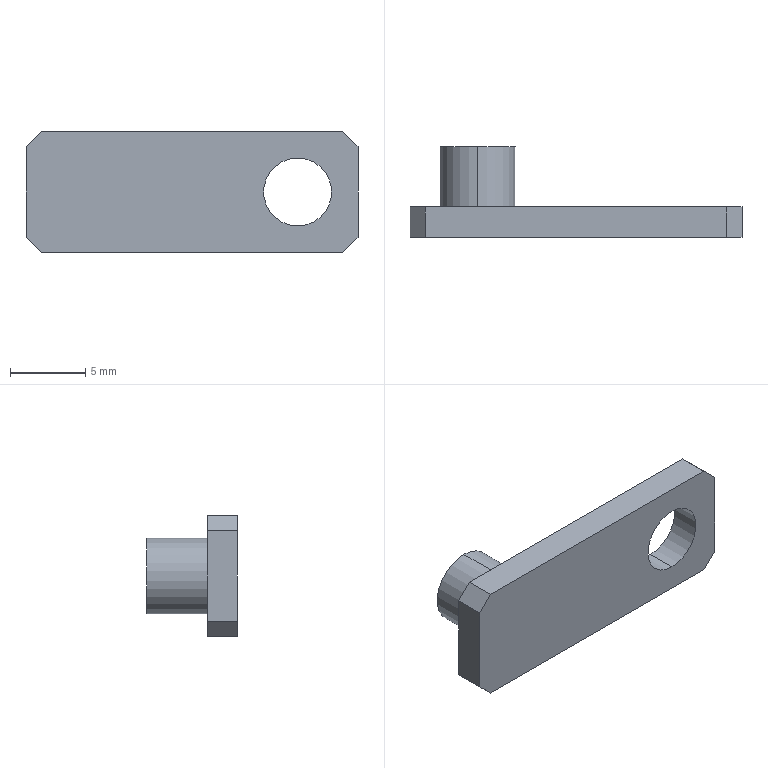Part | SolidWorks | features ICE 2, Chamfer 1, Extrusion 1 | 1 solid | 15 faces | box 22 x 6 x 8 mm | volume 394.731 mm3 | plane 11 | cylinder 4 | commonest cylinder face diameters 4.5 x2 5 x2
STEP:
#1=CARTESIAN_POINT('',(-6.5,6.,2.5));
#2=VERTEX_POINT('',#1);
#3=CARTESIAN_POINT('',(-6.5,6.,-2.5));
#4=VERTEX_POINT('',#3);
#5=CARTESIAN_POINT('',(-6.5,6.,0.));
#6=DIRECTION('',(0.,1.,0.));
#7=DIRECTION('',(0.,0.,1.));
#8=AXIS2_PLACEMENT_3D('',#5,#6,#7);
#9=CIRCLE('',#8,2.5);
#10=EDGE_CURVE('',#2,#4,#9,.T.);
#11=ORIENTED_EDGE('',*,*,#10,.F.);
#12=CARTESIAN_POINT('',(-6.5,2.,2.5));
#13=VERTEX_POINT('',#12);
#14=CARTESIAN_POINT('',(-6.5,6.,2.5));
#15=DIRECTION('',(0.,-1.,0.));
#16=VECTOR('',#15,1000.);
#17=LINE('',#14,#16);
#18=EDGE_CURVE('',#2,#13,#17,.T.);
#19=ORIENTED_EDGE('',*,*,#18,.T.);
#20=CARTESIAN_POINT('',(-6.5,2.,-2.5));
#21=VERTEX_POINT('',#20);
#22=CARTESIAN_POINT('',(-6.5,2.,0.));
#23=DIRECTION('',(0.,1.,0.));
#24=DIRECTION('',(0.,0.,-1.));
#25=AXIS2_PLACEMENT_3D('',#22,#23,#24);
#26=CIRCLE('',#25,2.5);
#27=EDGE_CURVE('',#13,#21,#26,.T.);
#28=ORIENTED_EDGE('',*,*,#27,.T.);
#29=CARTESIAN_POINT('',(-6.5,6.,-2.5));
#30=DIRECTION('',(0.,-1.,0.));
#31=VECTOR('',#30,1000.);
#32=LINE('',#29,#31);
#33=EDGE_CURVE('',#4,#21,#32,.T.);
#34=ORIENTED_EDGE('',*,*,#33,.F.);
#35=EDGE_LOOP('',(#11,#19,#28,#34));
#36=FACE_OUTER_BOUND('',#35,.T.);
#37=CARTESIAN_POINT('',(-6.5,6.,0.));
#38=DIRECTION('',(0.,-1.,0.));
#39=DIRECTION('',(0.,0.,-1.));
#40=AXIS2_PLACEMENT_3D('',#37,#38,#39);
#41=CYLINDRICAL_SURFACE('',#40,2.5);
#42=ADVANCED_FACE('',(#36),#41,.T.);
#43=CARTESIAN_POINT('',(7.,0.,-2.25));
#44=VERTEX_POINT('',#43);
#45=CARTESIAN_POINT('',(7.,0.,2.25));
#46=VERTEX_POINT('',#45);
#47=CARTESIAN_POINT('',(7.,0.,0.));
#48=DIRECTION('',(0.,1.,0.));
#49=DIRECTION('',(0.,0.,1.));
#50=AXIS2_PLACEMENT_3D('',#47,#48,#49);
#51=CIRCLE('',#50,2.25);
#52=EDGE_CURVE('',#44,#46,#51,.T.);
#53=ORIENTED_EDGE('',*,*,#52,.F.);
#54=CARTESIAN_POINT('',(7.,2.,-2.25));
#55=VERTEX_POINT('',#54);
#56=CARTESIAN_POINT('',(7.,0.,-2.25));
#57=DIRECTION('',(0.,1.,0.));
#58=VECTOR('',#57,1000.);
#59=LINE('',#56,#58);
#60=EDGE_CURVE('',#44,#55,#59,.T.);
#61=ORIENTED_EDGE('',*,*,#60,.T.);
#62=CARTESIAN_POINT('',(7.,2.,2.25));
#63=VERTEX_POINT('',#62);
#64=CARTESIAN_POINT('',(7.,2.,0.));
#65=DIRECTION('',(0.,1.,0.));
#66=DIRECTION('',(0.,0.,1.));
#67=AXIS2_PLACEMENT_3D('',#64,#65,#66);
#68=CIRCLE('',#67,2.25);
#69=EDGE_CURVE('',#55,#63,#68,.T.);
#70=ORIENTED_EDGE('',*,*,#69,.T.);
#71=CARTESIAN_POINT('',(7.,0.,2.25));
#72=DIRECTION('',(0.,1.,0.));
#73=VECTOR('',#72,1000.);
#74=LINE('',#71,#73);
#75=EDGE_CURVE('',#46,#63,#74,.T.);
#76=ORIENTED_EDGE('',*,*,#75,.F.);
#77=EDGE_LOOP('',(#53,#61,#70,#76));
#78=FACE_OUTER_BOUND('',#77,.T.);
#79=CARTESIAN_POINT('',(7.,0.,0.));
#80=DIRECTION('',(0.,1.,0.));
#81=DIRECTION('',(0.,0.,1.));
#82=AXIS2_PLACEMENT_3D('',#79,#80,#81);
#83=CYLINDRICAL_SURFACE('',#82,2.25);
#84=ADVANCED_FACE('',(#78),#83,.F.);
#85=CARTESIAN_POINT('',(11.,0.,3.));
#86=VERTEX_POINT('',#85);
#87=CARTESIAN_POINT('',(11.,0.,-3.));
#88=VERTEX_POINT('',#87);
#89=CARTESIAN_POINT('',(11.,0.,4.));
#90=DIRECTION('',(0.,0.,-1.));
#91=VECTOR('',#90,1000.);
#92=LINE('',#89,#91);
#93=EDGE_CURVE('',#86,#88,#92,.T.);
#94=ORIENTED_EDGE('',*,*,#93,.T.);
#95=CARTESIAN_POINT('',(11.,2.,-3.));
#96=VERTEX_POINT('',#95);
#97=CARTESIAN_POINT('',(11.,2.,-3.));
#98=DIRECTION('',(0.,1.,0.));
#99=VECTOR('',#98,1000.);
#100=LINE('',#97,#99);
#101=EDGE_CURVE('',#88,#96,#100,.T.);
#102=ORIENTED_EDGE('',*,*,#101,.T.);
#103=CARTESIAN_POINT('',(11.,2.,3.));
#104=VERTEX_POINT('',#103);
#105=CARTESIAN_POINT('',(11.,2.,4.));
#106=DIRECTION('',(0.,0.,-1.));
#107=VECTOR('',#106,1000.);
#108=LINE('',#105,#107);
#109=EDGE_CURVE('',#104,#96,#108,.T.);
#110=ORIENTED_EDGE('',*,*,#109,.F.);
#111=CARTESIAN_POINT('',(11.,2.,3.));
#112=DIRECTION('',(0.,-1.,0.));
#113=VECTOR('',#112,1000.);
#114=LINE('',#111,#113);
#115=EDGE_CURVE('',#104,#86,#114,.T.);
#116=ORIENTED_EDGE('',*,*,#115,.T.);
#117=EDGE_LOOP('',(#94,#102,#110,#116));
#118=FACE_OUTER_BOUND('',#117,.T.);
#119=CARTESIAN_POINT('',(11.,2.,4.));
#120=DIRECTION('',(-1.,0.,0.));
#121=DIRECTION('',(0.,0.,1.));
#122=AXIS2_PLACEMENT_3D('',#119,#120,#121);
#123=PLANE('',#122);
#124=ADVANCED_FACE('',(#118),#123,.F.);
#125=CARTESIAN_POINT('',(10.,2.,-4.));
#126=VERTEX_POINT('',#125);
#127=CARTESIAN_POINT('',(-10.,2.,-4.));
#128=VERTEX_POINT('',#127);
#129=CARTESIAN_POINT('',(-11.,2.,-4.));
#130=DIRECTION('',(-1.,0.,0.));
#131=VECTOR('',#130,1000.);
#132=LINE('',#129,#131);
#133=EDGE_CURVE('',#126,#128,#132,.T.);
#134=ORIENTED_EDGE('',*,*,#133,.F.);
#135=CARTESIAN_POINT('',(10.,0.,-4.));
#136=VERTEX_POINT('',#135);
#137=CARTESIAN_POINT('',(10.,2.,-4.));
#138=DIRECTION('',(0.,-1.,0.));
#139=VECTOR('',#138,1000.);
#140=LINE('',#137,#139);
#141=EDGE_CURVE('',#126,#136,#140,.T.);
#142=ORIENTED_EDGE('',*,*,#141,.T.);
#143=CARTESIAN_POINT('',(-10.,0.,-4.));
#144=VERTEX_POINT('',#143);
#145=CARTESIAN_POINT('',(-11.,0.,-4.));
#146=DIRECTION('',(-1.,0.,0.));
#147=VECTOR('',#146,1000.);
#148=LINE('',#145,#147);
#149=EDGE_CURVE('',#136,#144,#148,.T.);
#150=ORIENTED_EDGE('',*,*,#149,.T.);
#151=CARTESIAN_POINT('',(-10.,2.,-4.));
#152=DIRECTION('',(0.,1.,0.));
#153=VECTOR('',#152,1000.);
#154=LINE('',#151,#153);
#155=EDGE_CURVE('',#144,#128,#154,.T.);
#156=ORIENTED_EDGE('',*,*,#155,.T.);
#157=EDGE_LOOP('',(#134,#142,#150,#156));
#158=FACE_OUTER_BOUND('',#157,.T.);
#159=CARTESIAN_POINT('',(-11.,2.,-4.));
#160=DIRECTION('',(0.,0.,1.));
#161=DIRECTION('',(1.,0.,0.));
#162=AXIS2_PLACEMENT_3D('',#159,#160,#161);
#163=PLANE('',#162);
#164=ADVANCED_FACE('',(#158),#163,.F.);
#165=CARTESIAN_POINT('',(-11.,2.,-3.));
#166=VERTEX_POINT('',#165);
#167=CARTESIAN_POINT('',(-11.,2.,3.));
#168=VERTEX_POINT('',#167);
#169=CARTESIAN_POINT('',(-11.,2.,4.));
#170=DIRECTION('',(0.,0.,1.));
#171=VECTOR('',#170,1000.);
#172=LINE('',#169,#171);
#173=EDGE_CURVE('',#166,#168,#172,.T.);
#174=ORIENTED_EDGE('',*,*,#173,.F.);
#175=CARTESIAN_POINT('',(-11.,0.,-3.));
#176=VERTEX_POINT('',#175);
#177=CARTESIAN_POINT('',(-11.,2.,-3.));
#178=DIRECTION('',(0.,-1.,0.));
#179=VECTOR('',#178,1000.);
#180=LINE('',#177,#179);
#181=EDGE_CURVE('',#166,#176,#180,.T.);
#182=ORIENTED_EDGE('',*,*,#181,.T.);
#183=CARTESIAN_POINT('',(-11.,0.,3.));
#184=VERTEX_POINT('',#183);
#185=CARTESIAN_POINT('',(-11.,0.,4.));
#186=DIRECTION('',(0.,0.,1.));
#187=VECTOR('',#186,1000.);
#188=LINE('',#185,#187);
#189=EDGE_CURVE('',#176,#184,#188,.T.);
#190=ORIENTED_EDGE('',*,*,#189,.T.);
#191=CARTESIAN_POINT('',(-11.,2.,3.));
#192=DIRECTION('',(0.,1.,0.));
#193=VECTOR('',#192,1000.);
#194=LINE('',#191,#193);
#195=EDGE_CURVE('',#184,#168,#194,.T.);
#196=ORIENTED_EDGE('',*,*,#195,.T.);
#197=EDGE_LOOP('',(#174,#182,#190,#196));
#198=FACE_OUTER_BOUND('',#197,.T.);
#199=CARTESIAN_POINT('',(-11.,2.,4.));
#200=DIRECTION('',(1.,0.,0.));
#201=DIRECTION('',(0.,0.,-1.));
#202=AXIS2_PLACEMENT_3D('',#199,#200,#201);
#203=PLANE('',#202);
#204=ADVANCED_FACE('',(#198),#203,.F.);
#205=CARTESIAN_POINT('',(-10.,0.,4.));
#206=VERTEX_POINT('',#205);
#207=CARTESIAN_POINT('',(10.,0.,4.));
#208=VERTEX_POINT('',#207);
#209=CARTESIAN_POINT('',(-11.,0.,4.));
#210=DIRECTION('',(1.,0.,0.));
#211=VECTOR('',#210,1000.);
#212=LINE('',#209,#211);
#213=EDGE_CURVE('',#206,#208,#212,.T.);
#214=ORIENTED_EDGE('',*,*,#213,.T.);
#215=CARTESIAN_POINT('',(10.,2.,4.));
#216=VERTEX_POINT('',#215);
#217=CARTESIAN_POINT('',(10.,2.,4.));
#218=DIRECTION('',(0.,1.,0.));
#219=VECTOR('',#218,1000.);
#220=LINE('',#217,#219);
#221=EDGE_CURVE('',#208,#216,#220,.T.);
#222=ORIENTED_EDGE('',*,*,#221,.T.);
#223=CARTESIAN_POINT('',(-10.,2.,4.));
#224=VERTEX_POINT('',#223);
#225=CARTESIAN_POINT('',(-11.,2.,4.));
#226=DIRECTION('',(1.,0.,0.));
#227=VECTOR('',#226,1000.);
#228=LINE('',#225,#227);
#229=EDGE_CURVE('',#224,#216,#228,.T.);
#230=ORIENTED_EDGE('',*,*,#229,.F.);
#231=CARTESIAN_POINT('',(-10.,2.,4.));
#232=DIRECTION('',(0.,-1.,0.));
#233=VECTOR('',#232,1000.);
#234=LINE('',#231,#233);
#235=EDGE_CURVE('',#224,#206,#234,.T.);
#236=ORIENTED_EDGE('',*,*,#235,.T.);
#237=EDGE_LOOP('',(#214,#222,#230,#236));
#238=FACE_OUTER_BOUND('',#237,.T.);
#239=CARTESIAN_POINT('',(-11.,2.,4.));
#240=DIRECTION('',(0.,0.,-1.));
#241=DIRECTION('',(-1.,0.,0.));
#242=AXIS2_PLACEMENT_3D('',#239,#240,#241);
#243=PLANE('',#242);
#244=ADVANCED_FACE('',(#238),#243,.F.);
#245=CARTESIAN_POINT('',(-6.5,2.,0.));
#246=DIRECTION('',(0.,1.,0.));
#247=DIRECTION('',(0.,0.,-1.));
#248=AXIS2_PLACEMENT_3D('',#245,#246,#247);
#249=CIRCLE('',#248,2.5);
#250=EDGE_CURVE('',#21,#13,#249,.T.);
#251=ORIENTED_EDGE('',*,*,#250,.F.);
#252=ORIENTED_EDGE('',*,*,#27,.F.);
#253=EDGE_LOOP('',(#251,#252));
#254=FACE_BOUND('',#253,.T.);
#255=CARTESIAN_POINT('',(7.,2.,0.));
#256=DIRECTION('',(0.,1.,0.));
#257=DIRECTION('',(0.,0.,1.));
#258=AXIS2_PLACEMENT_3D('',#255,#256,#257);
#259=CIRCLE('',#258,2.25);
#260=EDGE_CURVE('',#63,#55,#259,.T.);
#261=ORIENTED_EDGE('',*,*,#260,.F.);
#262=ORIENTED_EDGE('',*,*,#69,.F.);
#263=EDGE_LOOP('',(#261,#262));
#264=FACE_BOUND('',#263,.T.);
#265=ORIENTED_EDGE('',*,*,#109,.T.);
#266=CARTESIAN_POINT('',(10.,2.,-4.));
#267=DIRECTION('',(-0.7071,0.,-0.7071));
#268=VECTOR('',#267,1000.);
#269=LINE('',#266,#268);
#270=EDGE_CURVE('',#96,#126,#269,.T.);
#271=ORIENTED_EDGE('',*,*,#270,.T.);
#272=ORIENTED_EDGE('',*,*,#133,.T.);
#273=CARTESIAN_POINT('',(-11.,2.,-3.));
#274=DIRECTION('',(-0.7071,0.,0.7071));
#275=VECTOR('',#274,1000.);
#276=LINE('',#273,#275);
#277=EDGE_CURVE('',#128,#166,#276,.T.);
#278=ORIENTED_EDGE('',*,*,#277,.T.);
#279=ORIENTED_EDGE('',*,*,#173,.T.);
#280=CARTESIAN_POINT('',(-10.,2.,4.));
#281=DIRECTION('',(0.7071,0.,0.7071));
#282=VECTOR('',#281,1000.);
#283=LINE('',#280,#282);
#284=EDGE_CURVE('',#168,#224,#283,.T.);
#285=ORIENTED_EDGE('',*,*,#284,.T.);
#286=ORIENTED_EDGE('',*,*,#229,.T.);
#287=CARTESIAN_POINT('',(11.,2.,3.));
#288=DIRECTION('',(0.7071,0.,-0.7071));
#289=VECTOR('',#288,1000.);
#290=LINE('',#287,#289);
#291=EDGE_CURVE('',#216,#104,#290,.T.);
#292=ORIENTED_EDGE('',*,*,#291,.T.);
#293=EDGE_LOOP('',(#265,#271,#272,#278,#279,#285,#286,#292));
#294=FACE_OUTER_BOUND('',#293,.T.);
#295=CARTESIAN_POINT('',(0.,2.,0.));
#296=DIRECTION('',(0.,-1.,0.));
#297=DIRECTION('',(0.,0.,-1.));
#298=AXIS2_PLACEMENT_3D('',#295,#296,#297);
#299=PLANE('',#298);
#300=ADVANCED_FACE('',(#254,#264,#294),#299,.F.);
#301=CARTESIAN_POINT('',(7.,0.,0.));
#302=DIRECTION('',(0.,1.,0.));
#303=DIRECTION('',(0.,0.,1.));
#304=AXIS2_PLACEMENT_3D('',#301,#302,#303);
#305=CIRCLE('',#304,2.25);
#306=EDGE_CURVE('',#46,#44,#305,.T.);
#307=ORIENTED_EDGE('',*,*,#306,.T.);
#308=ORIENTED_EDGE('',*,*,#52,.T.);
#309=EDGE_LOOP('',(#307,#308));
#310=FACE_BOUND('',#309,.T.);
#311=ORIENTED_EDGE('',*,*,#149,.F.);
#312=CARTESIAN_POINT('',(7.,0.,-7.));
#313=DIRECTION('',(0.7071,0.,0.7071));
#314=VECTOR('',#313,1000.);
#315=LINE('',#312,#314);
#316=EDGE_CURVE('',#136,#88,#315,.T.);
#317=ORIENTED_EDGE('',*,*,#316,.T.);
#318=ORIENTED_EDGE('',*,*,#93,.F.);
#319=CARTESIAN_POINT('',(7.,0.,7.));
#320=DIRECTION('',(-0.7071,0.,0.7071));
#321=VECTOR('',#320,1000.);
#322=LINE('',#319,#321);
#323=EDGE_CURVE('',#86,#208,#322,.T.);
#324=ORIENTED_EDGE('',*,*,#323,.T.);
#325=ORIENTED_EDGE('',*,*,#213,.F.);
#326=CARTESIAN_POINT('',(-7.,0.,7.));
#327=DIRECTION('',(-0.7071,0.,-0.7071));
#328=VECTOR('',#327,1000.);
#329=LINE('',#326,#328);
#330=EDGE_CURVE('',#206,#184,#329,.T.);
#331=ORIENTED_EDGE('',*,*,#330,.T.);
#332=ORIENTED_EDGE('',*,*,#189,.F.);
#333=CARTESIAN_POINT('',(-7.,0.,-7.));
#334=DIRECTION('',(0.7071,0.,-0.7071));
#335=VECTOR('',#334,1000.);
#336=LINE('',#333,#335);
#337=EDGE_CURVE('',#176,#144,#336,.T.);
#338=ORIENTED_EDGE('',*,*,#337,.T.);
#339=EDGE_LOOP('',(#311,#317,#318,#324,#325,#331,#332,#338));
#340=FACE_OUTER_BOUND('',#339,.T.);
#341=CARTESIAN_POINT('',(0.,0.,0.));
#342=DIRECTION('',(0.,-1.,0.));
#343=DIRECTION('',(0.,0.,-1.));
#344=AXIS2_PLACEMENT_3D('',#341,#342,#343);
#345=PLANE('',#344);
#346=ADVANCED_FACE('',(#310,#340),#345,.T.);
#347=ORIENTED_EDGE('',*,*,#60,.F.);
#348=ORIENTED_EDGE('',*,*,#306,.F.);
#349=ORIENTED_EDGE('',*,*,#75,.T.);
#350=ORIENTED_EDGE('',*,*,#260,.T.);
#351=EDGE_LOOP('',(#347,#348,#349,#350));
#352=FACE_OUTER_BOUND('',#351,.T.);
#353=CARTESIAN_POINT('',(7.,0.,0.));
#354=DIRECTION('',(0.,1.,0.));
#355=DIRECTION('',(0.,0.,1.));
#356=AXIS2_PLACEMENT_3D('',#353,#354,#355);
#357=CYLINDRICAL_SURFACE('',#356,2.25);
#358=ADVANCED_FACE('',(#352),#357,.F.);
#359=ORIENTED_EDGE('',*,*,#18,.F.);
#360=CARTESIAN_POINT('',(-6.5,6.,0.));
#361=DIRECTION('',(0.,1.,0.));
#362=DIRECTION('',(0.,0.,1.));
#363=AXIS2_PLACEMENT_3D('',#360,#361,#362);
#364=CIRCLE('',#363,2.5);
#365=EDGE_CURVE('',#4,#2,#364,.T.);
#366=ORIENTED_EDGE('',*,*,#365,.F.);
#367=ORIENTED_EDGE('',*,*,#33,.T.);
#368=ORIENTED_EDGE('',*,*,#250,.T.);
#369=EDGE_LOOP('',(#359,#366,#367,#368));
#370=FACE_OUTER_BOUND('',#369,.T.);
#371=CARTESIAN_POINT('',(-6.5,6.,0.));
#372=DIRECTION('',(0.,-1.,0.));
#373=DIRECTION('',(0.,0.,-1.));
#374=AXIS2_PLACEMENT_3D('',#371,#372,#373);
#375=CYLINDRICAL_SURFACE('',#374,2.5);
#376=ADVANCED_FACE('',(#370),#375,.T.);
#377=ORIENTED_EDGE('',*,*,#365,.T.);
#378=ORIENTED_EDGE('',*,*,#10,.T.);
#379=EDGE_LOOP('',(#377,#378));
#380=FACE_OUTER_BOUND('',#379,.T.);
#381=CARTESIAN_POINT('',(-6.5,6.,0.));
#382=DIRECTION('',(0.,1.,0.));
#383=DIRECTION('',(0.,0.,1.));
#384=AXIS2_PLACEMENT_3D('',#381,#382,#383);
#385=PLANE('',#384);
#386=ADVANCED_FACE('',(#380),#385,.T.);
#387=ORIENTED_EDGE('',*,*,#270,.F.);
#388=ORIENTED_EDGE('',*,*,#101,.F.);
#389=ORIENTED_EDGE('',*,*,#316,.F.);
#390=ORIENTED_EDGE('',*,*,#141,.F.);
#391=EDGE_LOOP('',(#387,#388,#389,#390));
#392=FACE_OUTER_BOUND('',#391,.T.);
#393=CARTESIAN_POINT('',(10.,2.,-4.));
#394=DIRECTION('',(-0.7071,0.,0.7071));
#395=DIRECTION('',(0.,-1.,0.));
#396=AXIS2_PLACEMENT_3D('',#393,#394,#395);
#397=PLANE('',#396);
#398=ADVANCED_FACE('',(#392),#397,.F.);
#399=ORIENTED_EDGE('',*,*,#291,.F.);
#400=ORIENTED_EDGE('',*,*,#221,.F.);
#401=ORIENTED_EDGE('',*,*,#323,.F.);
#402=ORIENTED_EDGE('',*,*,#115,.F.);
#403=EDGE_LOOP('',(#399,#400,#401,#402));
#404=FACE_OUTER_BOUND('',#403,.T.);
#405=CARTESIAN_POINT('',(11.,2.,3.));
#406=DIRECTION('',(-0.7071,0.,-0.7071));
#407=DIRECTION('',(0.,-1.,0.));
#408=AXIS2_PLACEMENT_3D('',#405,#406,#407);
#409=PLANE('',#408);
#410=ADVANCED_FACE('',(#404),#409,.F.);
#411=ORIENTED_EDGE('',*,*,#277,.F.);
#412=ORIENTED_EDGE('',*,*,#155,.F.);
#413=ORIENTED_EDGE('',*,*,#337,.F.);
#414=ORIENTED_EDGE('',*,*,#181,.F.);
#415=EDGE_LOOP('',(#411,#412,#413,#414));
#416=FACE_OUTER_BOUND('',#415,.T.);
#417=CARTESIAN_POINT('',(-11.,2.,-3.));
#418=DIRECTION('',(0.7071,0.,0.7071));
#419=DIRECTION('',(0.,-1.,0.));
#420=AXIS2_PLACEMENT_3D('',#417,#418,#419);
#421=PLANE('',#420);
#422=ADVANCED_FACE('',(#416),#421,.F.);
#423=ORIENTED_EDGE('',*,*,#284,.F.);
#424=ORIENTED_EDGE('',*,*,#195,.F.);
#425=ORIENTED_EDGE('',*,*,#330,.F.);
#426=ORIENTED_EDGE('',*,*,#235,.F.);
#427=EDGE_LOOP('',(#423,#424,#425,#426));
#428=FACE_OUTER_BOUND('',#427,.T.);
#429=CARTESIAN_POINT('',(-10.,2.,4.));
#430=DIRECTION('',(0.7071,0.,-0.7071));
#431=DIRECTION('',(0.,-1.,0.));
#432=AXIS2_PLACEMENT_3D('',#429,#430,#431);
#433=PLANE('',#432);
#434=ADVANCED_FACE('',(#428),#433,.F.);
#435=CLOSED_SHELL('',(#42,#84,#124,#164,#204,#244,#300,#346,#358,#376,#386,#398,#410,#422,#434));
#436=MANIFOLD_SOLID_BREP('',#435);
#437=CARTESIAN_POINT('',(0.,0.,0.));
#438=DIRECTION('',(0.,0.,1.));
#439=DIRECTION('',(1.,0.,0.));
#440=AXIS2_PLACEMENT_3D('',#437,#438,#439);
#441=(LENGTH_UNIT()NAMED_UNIT(*)SI_UNIT(.MILLI.,.METRE.));
#442=UNCERTAINTY_MEASURE_WITH_UNIT(LENGTH_MEASURE(0.00001),#441,'','');
#443=(NAMED_UNIT(*)PLANE_ANGLE_UNIT()SI_UNIT($,.RADIAN.));
#444=(NAMED_UNIT(*)SI_UNIT($,.STERADIAN.)SOLID_ANGLE_UNIT());
#445=(GEOMETRIC_REPRESENTATION_CONTEXT(3)GLOBAL_UNCERTAINTY_ASSIGNED_CONTEXT((#442))GLOBAL_UNIT_ASSIGNED_CONTEXT((#441,#443,#444))REPRESENTATION_CONTEXT('',''));
#446=ADVANCED_BREP_SHAPE_REPRESENTATION('',(#436,#440),#445);